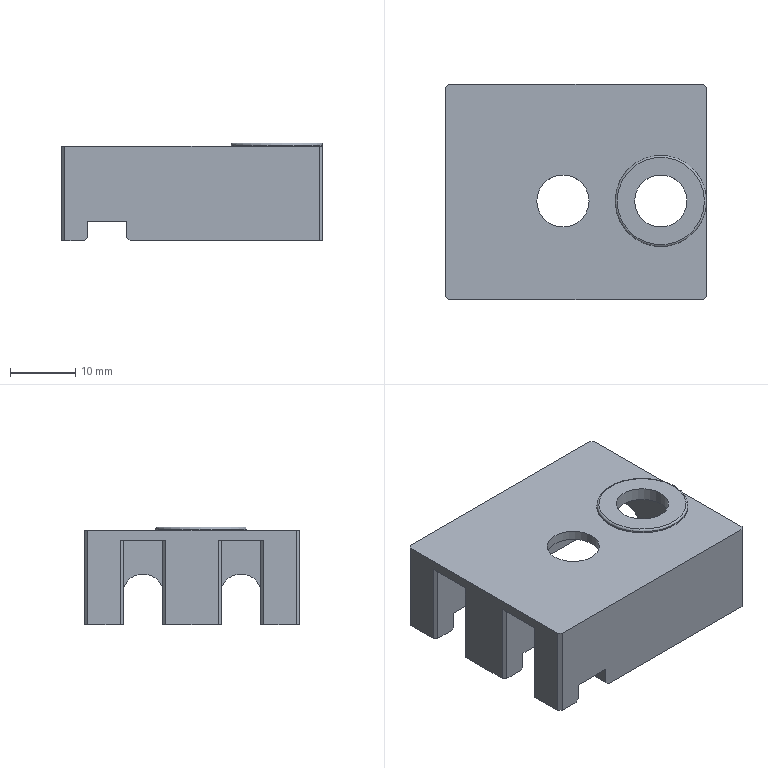Part | 1 solid | 72 faces | box 40 x 33 x 15 mm | volume 6484 mm3 | plane 52 | cylinder 16 | cone 3 | torus 1 | commonest cylinder face diameters 1 x8 2.459 x3 6.4 x2 8 x2 14 x1